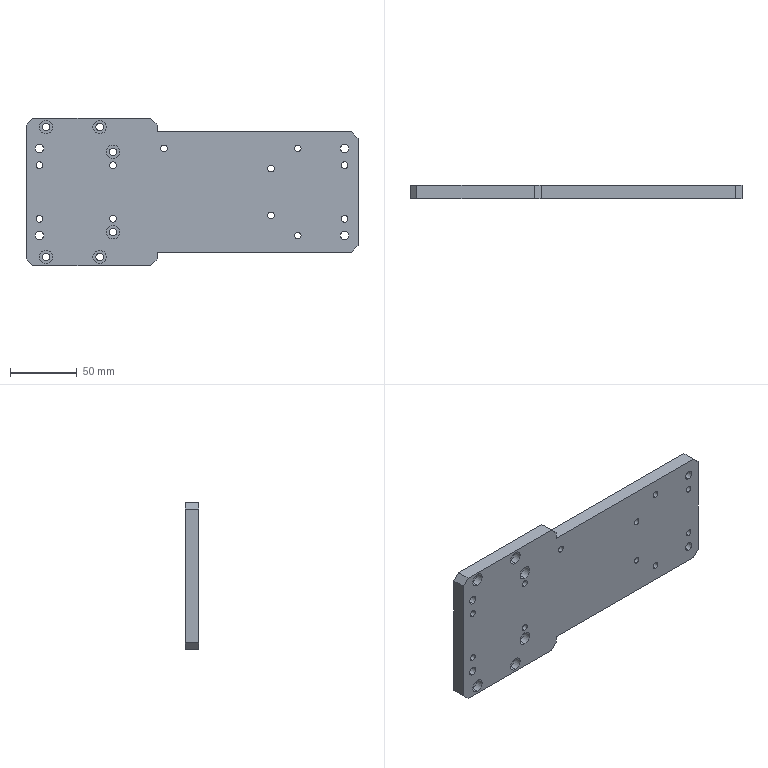Part | STEP file | PN_0028 | 1 solid | 76 faces | box 248 x 10 x 110 mm | volume 235264 mm3 | cylinder 54 | plane 22 | commonest cylinder face diameters 5 x22 5.5 x12 10 x12 6.5 x8